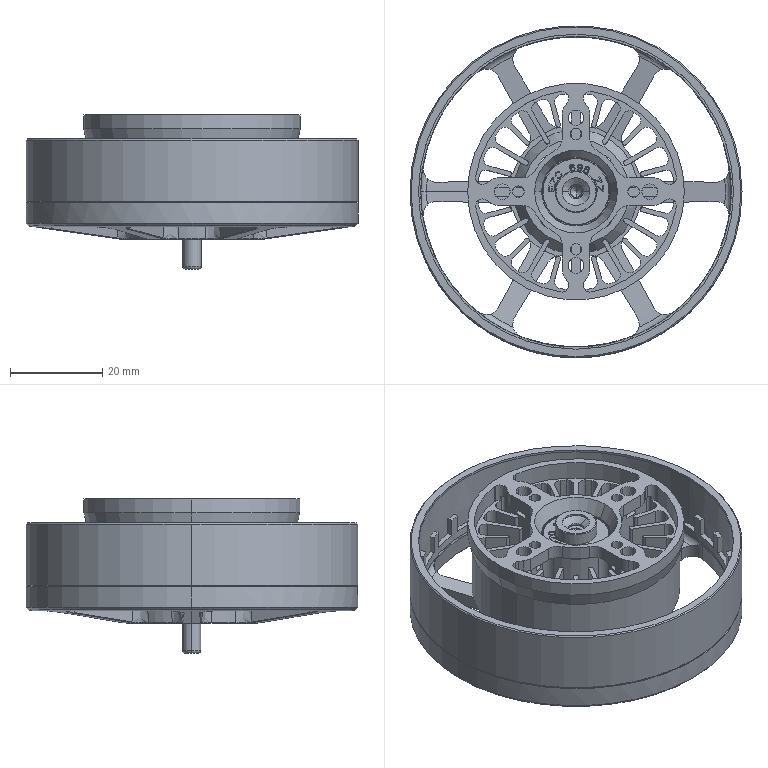Part | SolidWorks | features MBimport 1 | 1 solid | 1866 faces | box 72 x 72 x 33.4 mm | volume 24620 mm3 | plane 1365 | cylinder 313 | cone 87 | spline 73 | torus 28 | commonest cylinder face diameters 2.5 x77 3 x52 1 x38 6 x38 42.6 x24 3.4 x12